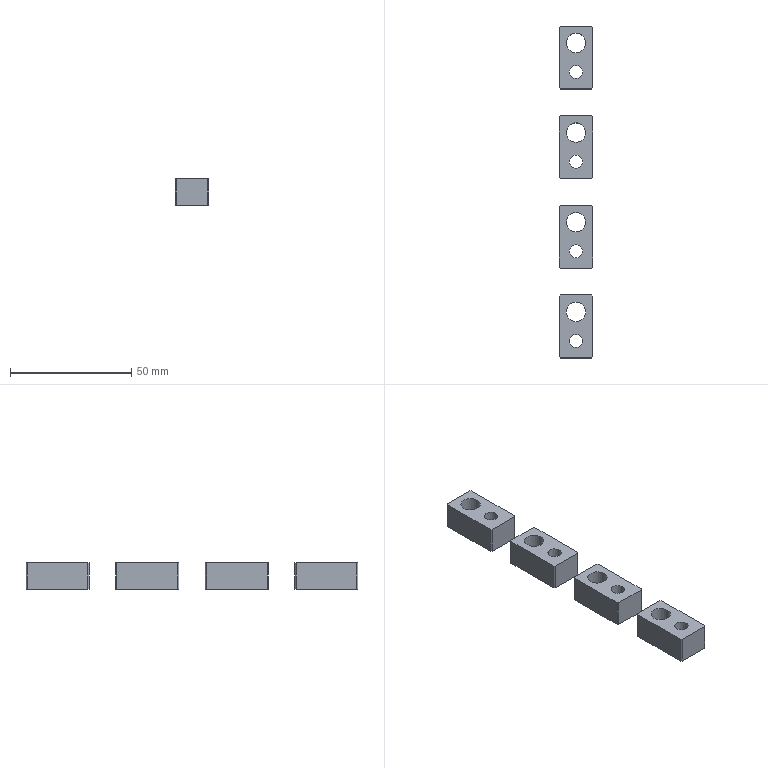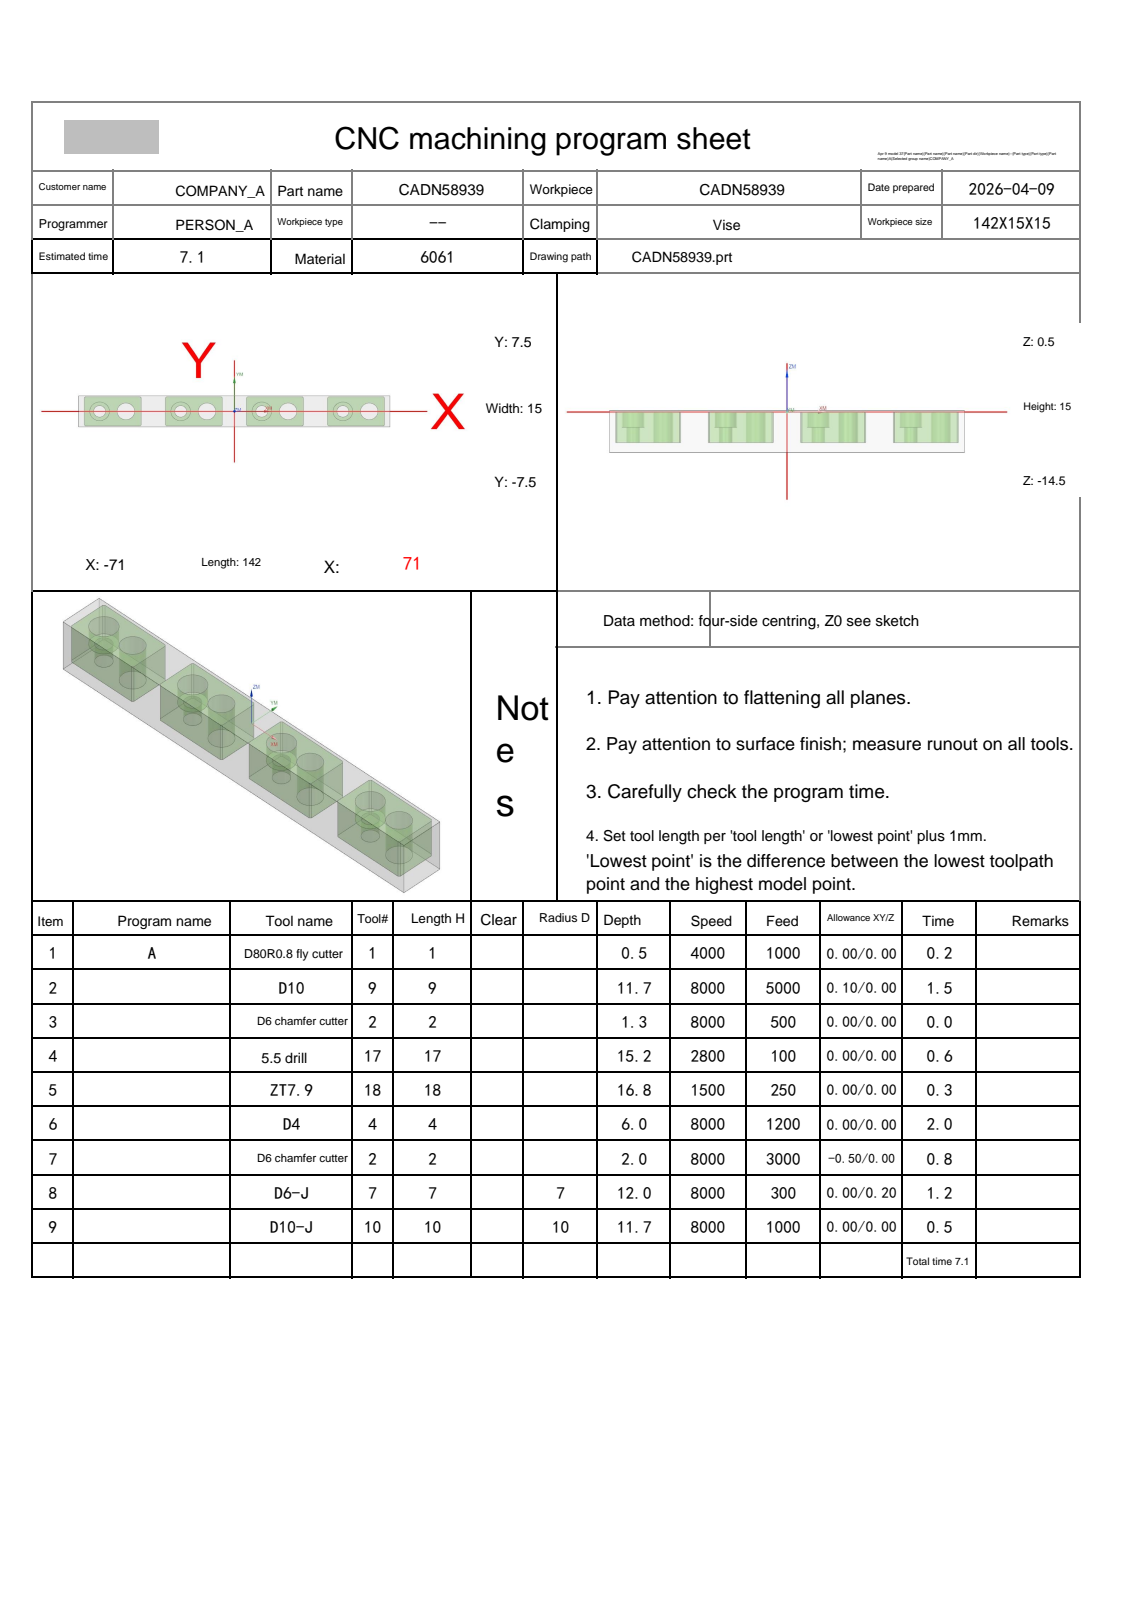NC program | NX | posted by the shop | part box 14 x 137 x 11 mm
Lines 1 to 1840 of 2072, first 1206 of 1838 lines:
%
O0001
(Machine time: 8.91 MIN)
(===Total Tool:8===)
(T1=D80R0.8 fly cutter D=80.  R=0.8  D-  H01 Z=-0.   )
(T9=D10     D=10.  R=0.   D-  H09 Z=-11.2 )
(T2=D6 chamfer cutter   D=6.   R=0.   D-  H02 Z=-1.5  )
(T17=5.5 drill  D=5.5  DR_a=118 D-  H17 Z=-14.65)
(T18=ZT7.9  D=7.9  DR_a=120 D-  H18 Z=-16.28)
(T4=D4      D=4.   R=0.   D4  H04 Z=-5.5  )
(T7=D6-J    D=6.   R=0.   D7  H07 Z=-11.5 )
(T10=D10-J  D=10.  R=0.   D10 H10 Z=-11.2 )
G80 G90 G17 G49 G40
G91 G28 Z0
M01
N1 T01 M06
(D80R0.8 fly cutter  D=80. R=0.8 H=01 ce=0.00 di=0.00)
G00 G90 G54 X-113.5 Y0.0 M03 S4000
G43 H01 Z20.
M08
Z2.
G01 Z0.0 F1000.
X-108.5
X108.5
X113.5
Z2.
G00 Z20.
G91 G28 Z0.0
M05
M09
G91 G28 Z0.0
M01
N2 T09 M06
(D10  D=10. R=0. H=09 ce=0.10 di=0.00)
G00 G90 G54 X18.5 Y12.1 M03 S8000
G43 H09 Z20.
M08
Z.5
G01 X31. Z.412 F5000.
G02 X34.606 Y10.606 Z.384 I0.0 J-5.1
G01 X35.106 Y10.106 Z.379
G02 X36.6 Y6.5 Z.351 I-3.606 J-3.606
G01 Y-6.5 Z.259
G02 X35.106 Y-10.106 Z.231 I-5.1 J0.0
G01 X34.606 Y-10.606 Z.226
G02 X31. Y-12.1 Z.198 I-3.606 J3.606
G01 X6. Z.022
G02 X2.394 Y-10.606 Z-.006 I0.0 J5.1
G01 X1.894 Y-10.106 Z-.011
G02 X.4 Y-6.5 Z-.039 I3.606 J3.606
G01 Y6.5 Z-.131
G02 X1.894 Y10.106 Z-.159 I5.1 J0.0
G01 X2.394 Y10.606 Z-.164
G02 X6. Y12.1 Z-.192 I3.606 J-3.606
G01 X31. Z-.368
G02 X34.606 Y10.606 Z-.396 I0.0 J-5.1
G01 X35.106 Y10.106 Z-.401
G02 X36.6 Y6.5 Z-.429 I-3.606 J-3.606
G01 Y-6.5 Z-.521
G02 X35.106 Y-10.106 Z-.549 I-5.1 J0.0
G01 X34.606 Y-10.606 Z-.554
G02 X31. Y-12.1 Z-.582 I-3.606 J3.606
G01 X6. Z-.758
G02 X2.394 Y-10.606 Z-.786 I0.0 J5.1
G01 X1.894 Y-10.106 Z-.791
G02 X.4 Y-6.5 Z-.819 I3.606 J3.606
G01 Y6.5 Z-.911
G02 X1.894 Y10.106 Z-.939 I5.1 J0.0
G01 X2.394 Y10.606 Z-.944
G02 X6. Y12.1 Z-.972 I3.606 J-3.606
G01 X31. Z-1.148
G02 X34.606 Y10.606 Z-1.176 I0.0 J-5.1
G01 X35.106 Y10.106 Z-1.181
G02 X36.6 Y6.5 Z-1.209 I-3.606 J-3.606
G01 Y-6.5 Z-1.301
G02 X35.106 Y-10.106 Z-1.329 I-5.1 J0.0
G01 X34.606 Y-10.606 Z-1.334
G02 X31. Y-12.1 Z-1.362 I-3.606 J3.606
G01 X6. Z-1.538
G02 X2.394 Y-10.606 Z-1.566 I0.0 J5.1
G01 X1.894 Y-10.106 Z-1.571
G02 X.4 Y-6.5 Z-1.599 I3.606 J3.606
G01 Y6.5 Z-1.691
G02 X1.894 Y10.106 Z-1.719 I5.1 J0.0
G01 X2.394 Y10.606 Z-1.724
G02 X6. Y12.1 Z-1.752 I3.606 J-3.606
G01 X31. Z-1.928
G02 X34.606 Y10.606 Z-1.956 I0.0 J-5.1
G01 X35.106 Y10.106 Z-1.961
G02 X36.6 Y6.5 Z-1.989 I-3.606 J-3.606
G01 Y-6.5 Z-2.081
G02 X35.106 Y-10.106 Z-2.109 I-5.1 J0.0
G01 X34.606 Y-10.606 Z-2.114
G02 X31. Y-12.1 Z-2.142 I-3.606 J3.606
G01 X6. Z-2.318
G02 X2.394 Y-10.606 Z-2.346 I0.0 J5.1
G01 X1.894 Y-10.106 Z-2.351
G02 X.4 Y-6.5 Z-2.379 I3.606 J3.606
G01 Y6.5 Z-2.471
G02 X1.894 Y10.106 Z-2.499 I5.1 J0.0
G01 X2.394 Y10.606 Z-2.504
G02 X6. Y12.1 Z-2.532 I3.606 J-3.606
G01 X31. Z-2.708
G02 X34.606 Y10.606 Z-2.736 I0.0 J-5.1
G01 X35.106 Y10.106 Z-2.741
G02 X36.6 Y6.5 Z-2.769 I-3.606 J-3.606
G01 Y-6.5 Z-2.861
G02 X35.106 Y-10.106 Z-2.889 I-5.1 J0.0
G01 X34.606 Y-10.606 Z-2.894
G02 X31. Y-12.1 Z-2.922 I-3.606 J3.606
G01 X6. Z-3.098
G02 X2.394 Y-10.606 Z-3.126 I0.0 J5.1
G01 X1.894 Y-10.106 Z-3.131
G02 X.4 Y-6.5 Z-3.159 I3.606 J3.606
G01 Y6.5 Z-3.251
G02 X1.894 Y10.106 Z-3.279 I5.1 J0.0
G01 X2.394 Y10.606 Z-3.284
G02 X6. Y12.1 Z-3.312 I3.606 J-3.606
G01 X31. Z-3.488
G02 X34.606 Y10.606 Z-3.516 I0.0 J-5.1
G01 X35.106 Y10.106 Z-3.521
G02 X36.6 Y6.5 Z-3.549 I-3.606 J-3.606
G01 Y-6.5 Z-3.641
G02 X35.106 Y-10.106 Z-3.669 I-5.1 J0.0
G01 X34.606 Y-10.606 Z-3.674
G02 X31. Y-12.1 Z-3.702 I-3.606 J3.606
G01 X6. Z-3.878
G02 X2.394 Y-10.606 Z-3.906 I0.0 J5.1
G01 X1.894 Y-10.106 Z-3.911
G02 X.4 Y-6.5 Z-3.939 I3.606 J3.606
G01 Y6.5 Z-4.031
G02 X1.894 Y10.106 Z-4.059 I5.1 J0.0
G01 X2.394 Y10.606 Z-4.064
G02 X6. Y12.1 Z-4.092 I3.606 J-3.606
G01 X31. Z-4.268
G02 X34.606 Y10.606 Z-4.296 I0.0 J-5.1
G01 X35.106 Y10.106 Z-4.301
G02 X36.6 Y6.5 Z-4.329 I-3.606 J-3.606
G01 Y-6.5 Z-4.421
G02 X35.106 Y-10.106 Z-4.449 I-5.1 J0.0
G01 X34.606 Y-10.606 Z-4.454
G02 X31. Y-12.1 Z-4.482 I-3.606 J3.606
G01 X6. Z-4.658
G02 X2.394 Y-10.606 Z-4.686 I0.0 J5.1
G01 X1.894 Y-10.106 Z-4.691
G02 X.4 Y-6.5 Z-4.719 I3.606 J3.606
G01 Y6.5 Z-4.811
G02 X1.894 Y10.106 Z-4.839 I5.1 J0.0
G01 X2.394 Y10.606 Z-4.844
G02 X6. Y12.1 Z-4.872 I3.606 J-3.606
G01 X31. Z-5.048
G02 X34.606 Y10.606 Z-5.076 I0.0 J-5.1
G01 X35.106 Y10.106 Z-5.081
G02 X36.6 Y6.5 Z-5.109 I-3.606 J-3.606
G01 Y-6.5 Z-5.201
G02 X35.106 Y-10.106 Z-5.229 I-5.1 J0.0
G01 X34.606 Y-10.606 Z-5.234
G02 X31. Y-12.1 Z-5.262 I-3.606 J3.606
G01 X6. Z-5.438
G02 X2.394 Y-10.606 Z-5.466 I0.0 J5.1
G01 X1.894 Y-10.106 Z-5.471
G02 X.4 Y-6.5 Z-5.499 I3.606 J3.606
G01 Y6.5 Z-5.591
G02 X1.894 Y10.106 Z-5.619 I5.1 J0.0
G01 X2.394 Y10.606 Z-5.624
G02 X6. Y12.1 Z-5.652 I3.606 J-3.606
G01 X31. Z-5.828
G02 X34.606 Y10.606 Z-5.856 I0.0 J-5.1
G01 X35.106 Y10.106 Z-5.861
G02 X36.6 Y6.5 Z-5.889 I-3.606 J-3.606
G01 Y-6.5 Z-5.981
G02 X35.106 Y-10.106 Z-6.009 I-5.1 J0.0
G01 X34.606 Y-10.606 Z-6.014
G02 X31. Y-12.1 Z-6.042 I-3.606 J3.606
G01 X6. Z-6.218
G02 X2.394 Y-10.606 Z-6.246 I0.0 J5.1
G01 X1.894 Y-10.106 Z-6.251
G02 X.4 Y-6.5 Z-6.279 I3.606 J3.606
G01 Y6.5 Z-6.371
G02 X1.894 Y10.106 Z-6.399 I5.1 J0.0
G01 X2.394 Y10.606 Z-6.404
G02 X6. Y12.1 Z-6.432 I3.606 J-3.606
G01 X31. Z-6.608
G02 X34.606 Y10.606 Z-6.636 I0.0 J-5.1
G01 X35.106 Y10.106 Z-6.641
G02 X36.6 Y6.5 Z-6.669 I-3.606 J-3.606
G01 Y-6.5 Z-6.761
G02 X35.106 Y-10.106 Z-6.789 I-5.1 J0.0
G01 X34.606 Y-10.606 Z-6.794
G02 X31. Y-12.1 Z-6.822 I-3.606 J3.606
G01 X6. Z-6.998
G02 X2.394 Y-10.606 Z-7.026 I0.0 J5.1
G01 X1.894 Y-10.106 Z-7.031
G02 X.4 Y-6.5 Z-7.059 I3.606 J3.606
G01 Y6.5 Z-7.151
G02 X1.894 Y10.106 Z-7.179 I5.1 J0.0
G01 X2.394 Y10.606 Z-7.184
G02 X6. Y12.1 Z-7.212 I3.606 J-3.606
G01 X31. Z-7.388
G02 X34.606 Y10.606 Z-7.416 I0.0 J-5.1
G01 X35.106 Y10.106 Z-7.421
G02 X36.6 Y6.5 Z-7.449 I-3.606 J-3.606
G01 Y-6.5 Z-7.541
G02 X35.106 Y-10.106 Z-7.569 I-5.1 J0.0
G01 X34.606 Y-10.606 Z-7.574
G02 X31. Y-12.1 Z-7.602 I-3.606 J3.606
G01 X6. Z-7.778
G02 X2.394 Y-10.606 Z-7.806 I0.0 J5.1
G01 X1.894 Y-10.106 Z-7.811
G02 X.4 Y-6.5 Z-7.839 I3.606 J3.606
G01 Y6.5 Z-7.931
G02 X1.894 Y10.106 Z-7.959 I5.1 J0.0
G01 X2.394 Y10.606 Z-7.964
G02 X6. Y12.1 Z-7.992 I3.606 J-3.606
G01 X31. Z-8.168
G02 X34.606 Y10.606 Z-8.196 I0.0 J-5.1
G01 X35.106 Y10.106 Z-8.201
G02 X36.6 Y6.5 Z-8.229 I-3.606 J-3.606
G01 Y-6.5 Z-8.321
G02 X35.106 Y-10.106 Z-8.349 I-5.1 J0.0
G01 X34.606 Y-10.606 Z-8.354
G02 X31. Y-12.1 Z-8.382 I-3.606 J3.606
G01 X6. Z-8.558
G02 X2.394 Y-10.606 Z-8.586 I0.0 J5.1
G01 X1.894 Y-10.106 Z-8.591
G02 X.4 Y-6.5 Z-8.619 I3.606 J3.606
G01 Y6.5 Z-8.711
G02 X1.894 Y10.106 Z-8.739 I5.1 J0.0
G01 X2.394 Y10.606 Z-8.744
G02 X6. Y12.1 Z-8.772 I3.606 J-3.606
G01 X31. Z-8.948
G02 X34.606 Y10.606 Z-8.976 I0.0 J-5.1
G01 X35.106 Y10.106 Z-8.981
G02 X36.6 Y6.5 Z-9.009 I-3.606 J-3.606
G01 Y-6.5 Z-9.101
G02 X35.106 Y-10.106 Z-9.129 I-5.1 J0.0
G01 X34.606 Y-10.606 Z-9.134
G02 X31. Y-12.1 Z-9.162 I-3.606 J3.606
G01 X6. Z-9.338
G02 X2.394 Y-10.606 Z-9.366 I0.0 J5.1
G01 X1.894 Y-10.106 Z-9.371
G02 X.4 Y-6.5 Z-9.399 I3.606 J3.606
G01 Y6.5 Z-9.491
G02 X1.894 Y10.106 Z-9.519 I5.1 J0.0
G01 X2.394 Y10.606 Z-9.524
G02 X6. Y12.1 Z-9.552 I3.606 J-3.606
G01 X31. Z-9.728
G02 X34.606 Y10.606 Z-9.756 I0.0 J-5.1
G01 X35.106 Y10.106 Z-9.761
G02 X36.6 Y6.5 Z-9.789 I-3.606 J-3.606
G01 Y-6.5 Z-9.881
G02 X35.106 Y-10.106 Z-9.909 I-5.1 J0.0
G01 X34.606 Y-10.606 Z-9.914
G02 X31. Y-12.1 Z-9.942 I-3.606 J3.606
G01 X6. Z-10.118
G02 X2.394 Y-10.606 Z-10.146 I0.0 J5.1
G01 X1.894 Y-10.106 Z-10.151
G02 X.4 Y-6.5 Z-10.179 I3.606 J3.606
G01 Y6.5 Z-10.271
G02 X1.894 Y10.106 Z-10.299 I5.1 J0.0
G01 X2.394 Y10.606 Z-10.304
G02 X6. Y12.1 Z-10.332 I3.606 J-3.606
G01 X31. Z-10.508
G02 X34.606 Y10.606 Z-10.536 I0.0 J-5.1
G01 X35.106 Y10.106 Z-10.541
G02 X36.6 Y6.5 Z-10.569 I-3.606 J-3.606
G01 Y-6.5 Z-10.661
G02 X35.106 Y-10.106 Z-10.689 I-5.1 J0.0
G01 X34.606 Y-10.606 Z-10.694
G02 X31. Y-12.1 Z-10.722 I-3.606 J3.606
G01 X6. Z-10.898
G02 X2.394 Y-10.606 Z-10.926 I0.0 J5.1
G01 X1.894 Y-10.106 Z-10.931
G02 X.4 Y-6.5 Z-10.959 I3.606 J3.606
G01 Y6.5 Z-11.051
G02 X1.894 Y10.106 Z-11.079 I5.1 J0.0
G01 X2.394 Y10.606 Z-11.084
G02 X6. Y12.1 Z-11.112 I3.606 J-3.606
G01 X18.5 Z-11.2
X31.
G02 X34.606 Y10.606 I0.0 J-5.1
G01 X35.106 Y10.106
G02 X36.6 Y6.5 I-3.606 J-3.606
G01 Y-6.5
G02 X35.106 Y-10.106 I-5.1 J0.0
G01 X34.606 Y-10.606
G02 X31. Y-12.1 I-3.606 J3.606
G01 X6.
G02 X2.394 Y-10.606 I0.0 J5.1
G01 X1.894 Y-10.106
G02 X.4 Y-6.5 I3.606 J3.606
G01 Y6.5
G02 X1.894 Y10.106 I5.1 J0.0
G01 X2.394 Y10.606
G02 X6. Y12.1 I3.606 J-3.606
G01 X18.5
X19.
Z-10.2
G00 Z20.
X-18.5
Z.5
G01 X-6. Z.412
G02 X-2.394 Y10.606 Z.384 I0.0 J-5.1
G01 X-1.894 Y10.106 Z.379
G02 X-.4 Y6.5 Z.351 I-3.606 J-3.606
G01 Y-6.5 Z.259
G02 X-1.894 Y-10.106 Z.231 I-5.1 J0.0
G01 X-2.394 Y-10.606 Z.226
G02 X-6. Y-12.1 Z.198 I-3.606 J3.606
G01 X-31. Z.022
G02 X-34.606 Y-10.606 Z-.006 I0.0 J5.1
G01 X-35.106 Y-10.106 Z-.011
G02 X-36.6 Y-6.5 Z-.039 I3.606 J3.606
G01 Y6.5 Z-.131
G02 X-35.106 Y10.106 Z-.159 I5.1 J0.0
G01 X-34.606 Y10.606 Z-.164
G02 X-31. Y12.1 Z-.192 I3.606 J-3.606
G01 X-6. Z-.368
G02 X-2.394 Y10.606 Z-.396 I0.0 J-5.1
G01 X-1.894 Y10.106 Z-.401
G02 X-.4 Y6.5 Z-.429 I-3.606 J-3.606
G01 Y-6.5 Z-.521
G02 X-1.894 Y-10.106 Z-.549 I-5.1 J0.0
G01 X-2.394 Y-10.606 Z-.554
G02 X-6. Y-12.1 Z-.582 I-3.606 J3.606
G01 X-31. Z-.758
G02 X-34.606 Y-10.606 Z-.786 I0.0 J5.1
G01 X-35.106 Y-10.106 Z-.791
G02 X-36.6 Y-6.5 Z-.819 I3.606 J3.606
G01 Y6.5 Z-.911
G02 X-35.106 Y10.106 Z-.939 I5.1 J0.0
G01 X-34.606 Y10.606 Z-.944
G02 X-31. Y12.1 Z-.972 I3.606 J-3.606
G01 X-6. Z-1.148
G02 X-2.394 Y10.606 Z-1.176 I0.0 J-5.1
G01 X-1.894 Y10.106 Z-1.181
G02 X-.4 Y6.5 Z-1.209 I-3.606 J-3.606
G01 Y-6.5 Z-1.301
G02 X-1.894 Y-10.106 Z-1.329 I-5.1 J0.0
G01 X-2.394 Y-10.606 Z-1.334
G02 X-6. Y-12.1 Z-1.362 I-3.606 J3.606
G01 X-31. Z-1.538
G02 X-34.606 Y-10.606 Z-1.566 I0.0 J5.1
G01 X-35.106 Y-10.106 Z-1.571
G02 X-36.6 Y-6.5 Z-1.599 I3.606 J3.606
G01 Y6.5 Z-1.691
G02 X-35.106 Y10.106 Z-1.719 I5.1 J0.0
G01 X-34.606 Y10.606 Z-1.724
G02 X-31. Y12.1 Z-1.752 I3.606 J-3.606
G01 X-6. Z-1.928
G02 X-2.394 Y10.606 Z-1.956 I0.0 J-5.1
G01 X-1.894 Y10.106 Z-1.961
G02 X-.4 Y6.5 Z-1.989 I-3.606 J-3.606
G01 Y-6.5 Z-2.081
G02 X-1.894 Y-10.106 Z-2.109 I-5.1 J0.0
G01 X-2.394 Y-10.606 Z-2.114
G02 X-6. Y-12.1 Z-2.142 I-3.606 J3.606
G01 X-31. Z-2.318
G02 X-34.606 Y-10.606 Z-2.346 I0.0 J5.1
G01 X-35.106 Y-10.106 Z-2.351
G02 X-36.6 Y-6.5 Z-2.379 I3.606 J3.606
G01 Y6.5 Z-2.471
G02 X-35.106 Y10.106 Z-2.499 I5.1 J0.0
G01 X-34.606 Y10.606 Z-2.504
G02 X-31. Y12.1 Z-2.532 I3.606 J-3.606
G01 X-6. Z-2.708
G02 X-2.394 Y10.606 Z-2.736 I0.0 J-5.1
G01 X-1.894 Y10.106 Z-2.741
G02 X-.4 Y6.5 Z-2.769 I-3.606 J-3.606
G01 Y-6.5 Z-2.861
G02 X-1.894 Y-10.106 Z-2.889 I-5.1 J0.0
G01 X-2.394 Y-10.606 Z-2.894
G02 X-6. Y-12.1 Z-2.922 I-3.606 J3.606
G01 X-31. Z-3.098
G02 X-34.606 Y-10.606 Z-3.126 I0.0 J5.1
G01 X-35.106 Y-10.106 Z-3.131
G02 X-36.6 Y-6.5 Z-3.159 I3.606 J3.606
G01 Y6.5 Z-3.251
G02 X-35.106 Y10.106 Z-3.279 I5.1 J0.0
G01 X-34.606 Y10.606 Z-3.284
G02 X-31. Y12.1 Z-3.312 I3.606 J-3.606
G01 X-6. Z-3.488
G02 X-2.394 Y10.606 Z-3.516 I0.0 J-5.1
G01 X-1.894 Y10.106 Z-3.521
G02 X-.4 Y6.5 Z-3.549 I-3.606 J-3.606
G01 Y-6.5 Z-3.641
G02 X-1.894 Y-10.106 Z-3.669 I-5.1 J0.0
G01 X-2.394 Y-10.606 Z-3.674
G02 X-6. Y-12.1 Z-3.702 I-3.606 J3.606
G01 X-31. Z-3.878
G02 X-34.606 Y-10.606 Z-3.906 I0.0 J5.1
G01 X-35.106 Y-10.106 Z-3.911
G02 X-36.6 Y-6.5 Z-3.939 I3.606 J3.606
G01 Y6.5 Z-4.031
G02 X-35.106 Y10.106 Z-4.059 I5.1 J0.0
G01 X-34.606 Y10.606 Z-4.064
G02 X-31. Y12.1 Z-4.092 I3.606 J-3.606
G01 X-6. Z-4.268
G02 X-2.394 Y10.606 Z-4.296 I0.0 J-5.1
G01 X-1.894 Y10.106 Z-4.301
G02 X-.4 Y6.5 Z-4.329 I-3.606 J-3.606
G01 Y-6.5 Z-4.421
G02 X-1.894 Y-10.106 Z-4.449 I-5.1 J0.0
G01 X-2.394 Y-10.606 Z-4.454
G02 X-6. Y-12.1 Z-4.482 I-3.606 J3.606
G01 X-31. Z-4.658
G02 X-34.606 Y-10.606 Z-4.686 I0.0 J5.1
G01 X-35.106 Y-10.106 Z-4.691
G02 X-36.6 Y-6.5 Z-4.719 I3.606 J3.606
G01 Y6.5 Z-4.811
G02 X-35.106 Y10.106 Z-4.839 I5.1 J0.0
G01 X-34.606 Y10.606 Z-4.844
G02 X-31. Y12.1 Z-4.872 I3.606 J-3.606
G01 X-6. Z-5.048
G02 X-2.394 Y10.606 Z-5.076 I0.0 J-5.1
G01 X-1.894 Y10.106 Z-5.081
G02 X-.4 Y6.5 Z-5.109 I-3.606 J-3.606
G01 Y-6.5 Z-5.201
G02 X-1.894 Y-10.106 Z-5.229 I-5.1 J0.0
G01 X-2.394 Y-10.606 Z-5.234
G02 X-6. Y-12.1 Z-5.262 I-3.606 J3.606
G01 X-31. Z-5.438
G02 X-34.606 Y-10.606 Z-5.466 I0.0 J5.1
G01 X-35.106 Y-10.106 Z-5.471
G02 X-36.6 Y-6.5 Z-5.499 I3.606 J3.606
G01 Y6.5 Z-5.591
G02 X-35.106 Y10.106 Z-5.619 I5.1 J0.0
G01 X-34.606 Y10.606 Z-5.624
G02 X-31. Y12.1 Z-5.652 I3.606 J-3.606
G01 X-6. Z-5.828
G02 X-2.394 Y10.606 Z-5.856 I0.0 J-5.1
G01 X-1.894 Y10.106 Z-5.861
G02 X-.4 Y6.5 Z-5.889 I-3.606 J-3.606
G01 Y-6.5 Z-5.981
G02 X-1.894 Y-10.106 Z-6.009 I-5.1 J0.0
G01 X-2.394 Y-10.606 Z-6.014
G02 X-6. Y-12.1 Z-6.042 I-3.606 J3.606
G01 X-31. Z-6.218
G02 X-34.606 Y-10.606 Z-6.246 I0.0 J5.1
G01 X-35.106 Y-10.106 Z-6.251
G02 X-36.6 Y-6.5 Z-6.279 I3.606 J3.606
G01 Y6.5 Z-6.371
G02 X-35.106 Y10.106 Z-6.399 I5.1 J0.0
G01 X-34.606 Y10.606 Z-6.404
G02 X-31. Y12.1 Z-6.432 I3.606 J-3.606
G01 X-6. Z-6.608
G02 X-2.394 Y10.606 Z-6.636 I0.0 J-5.1
G01 X-1.894 Y10.106 Z-6.641
G02 X-.4 Y6.5 Z-6.669 I-3.606 J-3.606
G01 Y-6.5 Z-6.761
G02 X-1.894 Y-10.106 Z-6.789 I-5.1 J0.0
G01 X-2.394 Y-10.606 Z-6.794
G02 X-6. Y-12.1 Z-6.822 I-3.606 J3.606
G01 X-31. Z-6.998
G02 X-34.606 Y-10.606 Z-7.026 I0.0 J5.1
G01 X-35.106 Y-10.106 Z-7.031
G02 X-36.6 Y-6.5 Z-7.059 I3.606 J3.606
G01 Y6.5 Z-7.151
G02 X-35.106 Y10.106 Z-7.179 I5.1 J0.0
G01 X-34.606 Y10.606 Z-7.184
G02 X-31. Y12.1 Z-7.212 I3.606 J-3.606
G01 X-6. Z-7.388
G02 X-2.394 Y10.606 Z-7.416 I0.0 J-5.1
G01 X-1.894 Y10.106 Z-7.421
G02 X-.4 Y6.5 Z-7.449 I-3.606 J-3.606
G01 Y-6.5 Z-7.541
G02 X-1.894 Y-10.106 Z-7.569 I-5.1 J0.0
G01 X-2.394 Y-10.606 Z-7.574
G02 X-6. Y-12.1 Z-7.602 I-3.606 J3.606
G01 X-31. Z-7.778
G02 X-34.606 Y-10.606 Z-7.806 I0.0 J5.1
G01 X-35.106 Y-10.106 Z-7.811
G02 X-36.6 Y-6.5 Z-7.839 I3.606 J3.606
G01 Y6.5 Z-7.931
G02 X-35.106 Y10.106 Z-7.959 I5.1 J0.0
G01 X-34.606 Y10.606 Z-7.964
G02 X-31. Y12.1 Z-7.992 I3.606 J-3.606
G01 X-6. Z-8.168
G02 X-2.394 Y10.606 Z-8.196 I0.0 J-5.1
G01 X-1.894 Y10.106 Z-8.201
G02 X-.4 Y6.5 Z-8.229 I-3.606 J-3.606
G01 Y-6.5 Z-8.321
G02 X-1.894 Y-10.106 Z-8.349 I-5.1 J0.0
G01 X-2.394 Y-10.606 Z-8.354
G02 X-6. Y-12.1 Z-8.382 I-3.606 J3.606
G01 X-31. Z-8.558
G02 X-34.606 Y-10.606 Z-8.586 I0.0 J5.1
G01 X-35.106 Y-10.106 Z-8.591
G02 X-36.6 Y-6.5 Z-8.619 I3.606 J3.606
G01 Y6.5 Z-8.711
G02 X-35.106 Y10.106 Z-8.739 I5.1 J0.0
G01 X-34.606 Y10.606 Z-8.744
G02 X-31. Y12.1 Z-8.772 I3.606 J-3.606
G01 X-6. Z-8.948
G02 X-2.394 Y10.606 Z-8.976 I0.0 J-5.1
G01 X-1.894 Y10.106 Z-8.981
G02 X-.4 Y6.5 Z-9.009 I-3.606 J-3.606
G01 Y-6.5 Z-9.101
G02 X-1.894 Y-10.106 Z-9.129 I-5.1 J0.0
G01 X-2.394 Y-10.606 Z-9.134
G02 X-6. Y-12.1 Z-9.162 I-3.606 J3.606
G01 X-31. Z-9.338
G02 X-34.606 Y-10.606 Z-9.366 I0.0 J5.1
G01 X-35.106 Y-10.106 Z-9.371
G02 X-36.6 Y-6.5 Z-9.399 I3.606 J3.606
G01 Y6.5 Z-9.491
G02 X-35.106 Y10.106 Z-9.519 I5.1 J0.0
G01 X-34.606 Y10.606 Z-9.524
G02 X-31. Y12.1 Z-9.552 I3.606 J-3.606
G01 X-6. Z-9.728
G02 X-2.394 Y10.606 Z-9.756 I0.0 J-5.1
G01 X-1.894 Y10.106 Z-9.761
G02 X-.4 Y6.5 Z-9.789 I-3.606 J-3.606
G01 Y-6.5 Z-9.881
G02 X-1.894 Y-10.106 Z-9.909 I-5.1 J0.0
G01 X-2.394 Y-10.606 Z-9.914
G02 X-6. Y-12.1 Z-9.942 I-3.606 J3.606
G01 X-31. Z-10.118
G02 X-34.606 Y-10.606 Z-10.146 I0.0 J5.1
G01 X-35.106 Y-10.106 Z-10.151
G02 X-36.6 Y-6.5 Z-10.179 I3.606 J3.606
G01 Y6.5 Z-10.271
G02 X-35.106 Y10.106 Z-10.299 I5.1 J0.0
G01 X-34.606 Y10.606 Z-10.304
G02 X-31. Y12.1 Z-10.332 I3.606 J-3.606
G01 X-6. Z-10.508
G02 X-2.394 Y10.606 Z-10.536 I0.0 J-5.1
G01 X-1.894 Y10.106 Z-10.541
G02 X-.4 Y6.5 Z-10.569 I-3.606 J-3.606
G01 Y-6.5 Z-10.661
G02 X-1.894 Y-10.106 Z-10.689 I-5.1 J0.0
G01 X-2.394 Y-10.606 Z-10.694
G02 X-6. Y-12.1 Z-10.722 I-3.606 J3.606
G01 X-31. Z-10.898
G02 X-34.606 Y-10.606 Z-10.926 I0.0 J5.1
G01 X-35.106 Y-10.106 Z-10.931
G02 X-36.6 Y-6.5 Z-10.959 I3.606 J3.606
G01 Y6.5 Z-11.051
G02 X-35.106 Y10.106 Z-11.079 I5.1 J0.0
G01 X-34.606 Y10.606 Z-11.084
G02 X-31. Y12.1 Z-11.112 I3.606 J-3.606
G01 X-18.5 Z-11.2
X-6.
G02 X-2.394 Y10.606 I0.0 J-5.1
G01 X-1.894 Y10.106
G02 X-.4 Y6.5 I-3.606 J-3.606
G01 Y-6.5
G02 X-1.894 Y-10.106 I-5.1 J0.0
G01 X-2.394 Y-10.606
G02 X-6. Y-12.1 I-3.606 J3.606
G01 X-31.
G02 X-34.606 Y-10.606 I0.0 J5.1
G01 X-35.106 Y-10.106
G02 X-36.6 Y-6.5 I3.606 J3.606
G01 Y6.5
G02 X-35.106 Y10.106 I5.1 J0.0
G01 X-34.606 Y10.606
G02 X-31. Y12.1 I3.606 J-3.606
G01 X-18.5
X-18.
Z-10.2
G00 Z20.
X-55.5
Z.5
G01 X-43. Z.412
G02 X-39.394 Y10.606 Z.384 I0.0 J-5.1
G01 X-38.894 Y10.106 Z.379
G02 X-37.4 Y6.5 Z.351 I-3.606 J-3.606
G01 Y-6.5 Z.259
G02 X-38.894 Y-10.106 Z.231 I-5.1 J0.0
G01 X-39.394 Y-10.606 Z.226
G02 X-43. Y-12.1 Z.198 I-3.606 J3.606
G01 X-68. Z.022
G02 X-71.606 Y-10.606 Z-.006 I0.0 J5.1
G01 X-72.106 Y-10.106 Z-.011
G02 X-73.6 Y-6.5 Z-.039 I3.606 J3.606
G01 Y6.5 Z-.131
G02 X-72.106 Y10.106 Z-.159 I5.1 J0.0
G01 X-71.606 Y10.606 Z-.164
G02 X-68. Y12.1 Z-.192 I3.606 J-3.606
G01 X-43. Z-.368
G02 X-39.394 Y10.606 Z-.396 I0.0 J-5.1
G01 X-38.894 Y10.106 Z-.401
G02 X-37.4 Y6.5 Z-.429 I-3.606 J-3.606
G01 Y-6.5 Z-.521
G02 X-38.894 Y-10.106 Z-.549 I-5.1 J0.0
G01 X-39.394 Y-10.606 Z-.554
G02 X-43. Y-12.1 Z-.582 I-3.606 J3.606
G01 X-68. Z-.758
G02 X-71.606 Y-10.606 Z-.786 I0.0 J5.1
G01 X-72.106 Y-10.106 Z-.791
G02 X-73.6 Y-6.5 Z-.819 I3.606 J3.606
G01 Y6.5 Z-.911
G02 X-72.106 Y10.106 Z-.939 I5.1 J0.0
G01 X-71.606 Y10.606 Z-.944
G02 X-68. Y12.1 Z-.972 I3.606 J-3.606
G01 X-43. Z-1.148
G02 X-39.394 Y10.606 Z-1.176 I0.0 J-5.1
G01 X-38.894 Y10.106 Z-1.181
G02 X-37.4 Y6.5 Z-1.209 I-3.606 J-3.606
G01 Y-6.5 Z-1.301
G02 X-38.894 Y-10.106 Z-1.329 I-5.1 J0.0
G01 X-39.394 Y-10.606 Z-1.334
G02 X-43. Y-12.1 Z-1.362 I-3.606 J3.606
G01 X-68. Z-1.538
G02 X-71.606 Y-10.606 Z-1.566 I0.0 J5.1
G01 X-72.106 Y-10.106 Z-1.571
G02 X-73.6 Y-6.5 Z-1.599 I3.606 J3.606
G01 Y6.5 Z-1.691
G02 X-72.106 Y10.106 Z-1.719 I5.1 J0.0
G01 X-71.606 Y10.606 Z-1.724
G02 X-68. Y12.1 Z-1.752 I3.606 J-3.606
G01 X-43. Z-1.928
G02 X-39.394 Y10.606 Z-1.956 I0.0 J-5.1
G01 X-38.894 Y10.106 Z-1.961
G02 X-37.4 Y6.5 Z-1.989 I-3.606 J-3.606
G01 Y-6.5 Z-2.081
G02 X-38.894 Y-10.106 Z-2.109 I-5.1 J0.0
G01 X-39.394 Y-10.606 Z-2.114
G02 X-43. Y-12.1 Z-2.142 I-3.606 J3.606
G01 X-68. Z-2.318
G02 X-71.606 Y-10.606 Z-2.346 I0.0 J5.1
G01 X-72.106 Y-10.106 Z-2.351
G02 X-73.6 Y-6.5 Z-2.379 I3.606 J3.606
G01 Y6.5 Z-2.471
G02 X-72.106 Y10.106 Z-2.499 I5.1 J0.0
G01 X-71.606 Y10.606 Z-2.504
G02 X-68. Y12.1 Z-2.532 I3.606 J-3.606
G01 X-43. Z-2.708
G02 X-39.394 Y10.606 Z-2.736 I0.0 J-5.1
G01 X-38.894 Y10.106 Z-2.741
G02 X-37.4 Y6.5 Z-2.769 I-3.606 J-3.606
G01 Y-6.5 Z-2.861
G02 X-38.894 Y-10.106 Z-2.889 I-5.1 J0.0
G01 X-39.394 Y-10.606 Z-2.894
G02 X-43. Y-12.1 Z-2.922 I-3.606 J3.606
G01 X-68. Z-3.098
G02 X-71.606 Y-10.606 Z-3.126 I0.0 J5.1
G01 X-72.106 Y-10.106 Z-3.131
G02 X-73.6 Y-6.5 Z-3.159 I3.606 J3.606
G01 Y6.5 Z-3.251
G02 X-72.106 Y10.106 Z-3.279 I5.1 J0.0
G01 X-71.606 Y10.606 Z-3.284
G02 X-68. Y12.1 Z-3.312 I3.606 J-3.606
G01 X-43. Z-3.488
G02 X-39.394 Y10.606 Z-3.516 I0.0 J-5.1
G01 X-38.894 Y10.106 Z-3.521
G02 X-37.4 Y6.5 Z-3.549 I-3.606 J-3.606
G01 Y-6.5 Z-3.641
G02 X-38.894 Y-10.106 Z-3.669 I-5.1 J0.0
G01 X-39.394 Y-10.606 Z-3.674
G02 X-43. Y-12.1 Z-3.702 I-3.606 J3.606
G01 X-68. Z-3.878
G02 X-71.606 Y-10.606 Z-3.906 I0.0 J5.1
G01 X-72.106 Y-10.106 Z-3.911
G02 X-73.6 Y-6.5 Z-3.939 I3.606 J3.606
G01 Y6.5 Z-4.031
G02 X-72.106 Y10.106 Z-4.059 I5.1 J0.0
G01 X-71.606 Y10.606 Z-4.064
G02 X-68. Y12.1 Z-4.092 I3.606 J-3.606
G01 X-43. Z-4.268
G02 X-39.394 Y10.606 Z-4.296 I0.0 J-5.1
G01 X-38.894 Y10.106 Z-4.301
G02 X-37.4 Y6.5 Z-4.329 I-3.606 J-3.606
G01 Y-6.5 Z-4.421
G02 X-38.894 Y-10.106 Z-4.449 I-5.1 J0.0
G01 X-39.394 Y-10.606 Z-4.454
G02 X-43. Y-12.1 Z-4.482 I-3.606 J3.606
G01 X-68. Z-4.658
G02 X-71.606 Y-10.606 Z-4.686 I0.0 J5.1
G01 X-72.106 Y-10.106 Z-4.691
G02 X-73.6 Y-6.5 Z-4.719 I3.606 J3.606
G01 Y6.5 Z-4.811
G02 X-72.106 Y10.106 Z-4.839 I5.1 J0.0
G01 X-71.606 Y10.606 Z-4.844
G02 X-68. Y12.1 Z-4.872 I3.606 J-3.606
G01 X-43. Z-5.048
G02 X-39.394 Y10.606 Z-5.076 I0.0 J-5.1
G01 X-38.894 Y10.106 Z-5.081
G02 X-37.4 Y6.5 Z-5.109 I-3.606 J-3.606
G01 Y-6.5 Z-5.201
G02 X-38.894 Y-10.106 Z-5.229 I-5.1 J0.0
G01 X-39.394 Y-10.606 Z-5.234
G02 X-43. Y-12.1 Z-5.262 I-3.606 J3.606
G01 X-68. Z-5.438
G02 X-71.606 Y-10.606 Z-5.466 I0.0 J5.1
G01 X-72.106 Y-10.106 Z-5.471
G02 X-73.6 Y-6.5 Z-5.499 I3.606 J3.606
G01 Y6.5 Z-5.591
G02 X-72.106 Y10.106 Z-5.619 I5.1 J0.0
G01 X-71.606 Y10.606 Z-5.624
G02 X-68. Y12.1 Z-5.652 I3.606 J-3.606
G01 X-43. Z-5.828
G02 X-39.394 Y10.606 Z-5.856 I0.0 J-5.1
G01 X-38.894 Y10.106 Z-5.861
G02 X-37.4 Y6.5 Z-5.889 I-3.606 J-3.606
G01 Y-6.5 Z-5.981
G02 X-38.894 Y-10.106 Z-6.009 I-5.1 J0.0
G01 X-39.394 Y-10.606 Z-6.014
G02 X-43. Y-12.1 Z-6.042 I-3.606 J3.606
G01 X-68. Z-6.218
G02 X-71.606 Y-10.606 Z-6.246 I0.0 J5.1
G01 X-72.106 Y-10.106 Z-6.251
G02 X-73.6 Y-6.5 Z-6.279 I3.606 J3.606
G01 Y6.5 Z-6.371
G02 X-72.106 Y10.106 Z-6.399 I5.1 J0.0
G01 X-71.606 Y10.606 Z-6.404
G02 X-68. Y12.1 Z-6.432 I3.606 J-3.606
G01 X-43. Z-6.608
G02 X-39.394 Y10.606 Z-6.636 I0.0 J-5.1
G01 X-38.894 Y10.106 Z-6.641
G02 X-37.4 Y6.5 Z-6.669 I-3.606 J-3.606
G01 Y-6.5 Z-6.761
G02 X-38.894 Y-10.106 Z-6.789 I-5.1 J0.0
G01 X-39.394 Y-10.606 Z-6.794
G02 X-43. Y-12.1 Z-6.822 I-3.606 J3.606
G01 X-68. Z-6.998
G02 X-71.606 Y-10.606 Z-7.026 I0.0 J5.1
G01 X-72.106 Y-10.106 Z-7.031
G02 X-73.6 Y-6.5 Z-7.059 I3.606 J3.606
G01 Y6.5 Z-7.151
G02 X-72.106 Y10.106 Z-7.179 I5.1 J0.0
G01 X-71.606 Y10.606 Z-7.184
G02 X-68. Y12.1 Z-7.212 I3.606 J-3.606
G01 X-43. Z-7.388
G02 X-39.394 Y10.606 Z-7.416 I0.0 J-5.1
G01 X-38.894 Y10.106 Z-7.421
G02 X-37.4 Y6.5 Z-7.449 I-3.606 J-3.606
G01 Y-6.5 Z-7.541
G02 X-38.894 Y-10.106 Z-7.569 I-5.1 J0.0
G01 X-39.394 Y-10.606 Z-7.574
G02 X-43. Y-12.1 Z-7.602 I-3.606 J3.606
G01 X-68. Z-7.778
G02 X-71.606 Y-10.606 Z-7.806 I0.0 J5.1
G01 X-72.106 Y-10.106 Z-7.811
G02 X-73.6 Y-6.5 Z-7.839 I3.606 J3.606
G01 Y6.5 Z-7.931
G02 X-72.106 Y10.106 Z-7.959 I5.1 J0.0
G01 X-71.606 Y10.606 Z-7.964
G02 X-68. Y12.1 Z-7.992 I3.606 J-3.606
G01 X-43. Z-8.168
G02 X-39.394 Y10.606 Z-8.196 I0.0 J-5.1
G01 X-38.894 Y10.106 Z-8.201
G02 X-37.4 Y6.5 Z-8.229 I-3.606 J-3.606
G01 Y-6.5 Z-8.321
G02 X-38.894 Y-10.106 Z-8.349 I-5.1 J0.0
G01 X-39.394 Y-10.606 Z-8.354
G02 X-43. Y-12.1 Z-8.382 I-3.606 J3.606
G01 X-68. Z-8.558
G02 X-71.606 Y-10.606 Z-8.586 I0.0 J5.1
G01 X-72.106 Y-10.106 Z-8.591
G02 X-73.6 Y-6.5 Z-8.619 I3.606 J3.606
G01 Y6.5 Z-8.711
G02 X-72.106 Y10.106 Z-8.739 I5.1 J0.0
G01 X-71.606 Y10.606 Z-8.744
G02 X-68. Y12.1 Z-8.772 I3.606 J-3.606
G01 X-43. Z-8.948
G02 X-39.394 Y10.606 Z-8.976 I0.0 J-5.1
G01 X-38.894 Y10.106 Z-8.981
G02 X-37.4 Y6.5 Z-9.009 I-3.606 J-3.606
G01 Y-6.5 Z-9.101
G02 X-38.894 Y-10.106 Z-9.129 I-5.1 J0.0
G01 X-39.394 Y-10.606 Z-9.134
G02 X-43. Y-12.1 Z-9.162 I-3.606 J3.606
G01 X-68. Z-9.338
G02 X-71.606 Y-10.606 Z-9.366 I0.0 J5.1
G01 X-72.106 Y-10.106 Z-9.371
G02 X-73.6 Y-6.5 Z-9.399 I3.606 J3.606
G01 Y6.5 Z-9.491
G02 X-72.106 Y10.106 Z-9.519 I5.1 J0.0
G01 X-71.606 Y10.606 Z-9.524
G02 X-68. Y12.1 Z-9.552 I3.606 J-3.606
G01 X-43. Z-9.728
G02 X-39.394 Y10.606 Z-9.756 I0.0 J-5.1
G01 X-38.894 Y10.106 Z-9.761
G02 X-37.4 Y6.5 Z-9.789 I-3.606 J-3.606
G01 Y-6.5 Z-9.881
G02 X-38.894 Y-10.106 Z-9.909 I-5.1 J0.0
G01 X-39.394 Y-10.606 Z-9.914
G02 X-43. Y-12.1 Z-9.942 I-3.606 J3.606
G01 X-68. Z-10.118
G02 X-71.606 Y-10.606 Z-10.146 I0.0 J5.1
G01 X-72.106 Y-10.106 Z-10.151
G02 X-73.6 Y-6.5 Z-10.179 I3.606 J3.606
G01 Y6.5 Z-10.271
G02 X-72.106 Y10.106 Z-10.299 I5.1 J0.0
G01 X-71.606 Y10.606 Z-10.304
G02 X-68. Y12.1 Z-10.332 I3.606 J-3.606
G01 X-43. Z-10.508
G02 X-39.394 Y10.606 Z-10.536 I0.0 J-5.1
G01 X-38.894 Y10.106 Z-10.541
G02 X-37.4 Y6.5 Z-10.569 I-3.606 J-3.606
G01 Y-6.5 Z-10.661
G02 X-38.894 Y-10.106 Z-10.689 I-5.1 J0.0
G01 X-39.394 Y-10.606 Z-10.694
G02 X-43. Y-12.1 Z-10.722 I-3.606 J3.606
G01 X-68. Z-10.898
G02 X-71.606 Y-10.606 Z-10.926 I0.0 J5.1
G01 X-72.106 Y-10.106 Z-10.931
G02 X-73.6 Y-6.5 Z-10.959 I3.606 J3.606
G01 Y6.5 Z-11.051
G02 X-72.106 Y10.106 Z-11.079 I5.1 J0.0
G01 X-71.606 Y10.606 Z-11.084
G02 X-68. Y12.1 Z-11.112 I3.606 J-3.606
G01 X-55.5 Z-11.2
X-43.
G02 X-39.394 Y10.606 I0.0 J-5.1
G01 X-38.894 Y10.106
G02 X-37.4 Y6.5 I-3.606 J-3.606
G01 Y-6.5
G02 X-38.894 Y-10.106 I-5.1 J0.0
G01 X-39.394 Y-10.606
G02 X-43. Y-12.1 I-3.606 J3.606
G01 X-68.
G02 X-71.606 Y-10.606 I0.0 J5.1
G01 X-72.106 Y-10.106
G02 X-73.6 Y-6.5 I3.606 J3.606
G01 Y6.5
G02 X-72.106 Y10.106 I5.1 J0.0
G01 X-71.606 Y10.606
G02 X-68. Y12.1 I3.606 J-3.606
G01 X-55.5
X-55.
Z-10.2
G00 Z20.
X55.5 Y-12.1
Z.5
G01 X43. Z.412
G02 X39.394 Y-10.606 Z.384 I0.0 J5.1
G01 X38.894 Y-10.106 Z.379
G02 X37.4 Y-6.5 Z.351 I3.606 J3.606
G01 Y6.5 Z.259
G02 X38.894 Y10.106 Z.231 I5.1 J0.0
G01 X39.394 Y10.606 Z.226
G02 X43. Y12.1 Z.198 I3.606 J-3.606
G01 X68. Z.022
G02 X71.606 Y10.606 Z-.006 I0.0 J-5.1
G01 X72.106 Y10.106 Z-.011
G02 X73.6 Y6.5 Z-.039 I-3.606 J-3.606
G01 Y-6.5 Z-.131
G02 X72.106 Y-10.106 Z-.159 I-5.1 J0.0
G01 X71.606 Y-10.606 Z-.164
G02 X68. Y-12.1 Z-.192 I-3.606 J3.606
G01 X43. Z-.368
G02 X39.394 Y-10.606 Z-.396 I0.0 J5.1
G01 X38.894 Y-10.106 Z-.401
G02 X37.4 Y-6.5 Z-.429 I3.606 J3.606
G01 Y6.5 Z-.521
G02 X38.894 Y10.106 Z-.549 I5.1 J0.0
G01 X39.394 Y10.606 Z-.554
G02 X43. Y12.1 Z-.582 I3.606 J-3.606
G01 X68. Z-.758
G02 X71.606 Y10.606 Z-.786 I0.0 J-5.1
G01 X72.106 Y10.106 Z-.791
G02 X73.6 Y6.5 Z-.819 I-3.606 J-3.606
G01 Y-6.5 Z-.911
G02 X72.106 Y-10.106 Z-.939 I-5.1 J0.0
G01 X71.606 Y-10.606 Z-.944
G02 X68. Y-12.1 Z-.972 I-3.606 J3.606
G01 X43. Z-1.148
G02 X39.394 Y-10.606 Z-1.176 I0.0 J5.1
G01 X38.894 Y-10.106 Z-1.181
G02 X37.4 Y-6.5 Z-1.209 I3.606 J3.606
G01 Y6.5 Z-1.301
G02 X38.894 Y10.106 Z-1.329 I5.1 J0.0
G01 X39.394 Y10.606 Z-1.334
G02 X43. Y12.1 Z-1.362 I3.606 J-3.606
G01 X68. Z-1.538
G02 X71.606 Y10.606 Z-1.566 I0.0 J-5.1
G01 X72.106 Y10.106 Z-1.571
G02 X73.6 Y6.5 Z-1.599 I-3.606 J-3.606
G01 Y-6.5 Z-1.691
G02 X72.106 Y-10.106 Z-1.719 I-5.1 J0.0
G01 X71.606 Y-10.606 Z-1.724
G02 X68. Y-12.1 Z-1.752 I-3.606 J3.606
G01 X43. Z-1.928
G02 X39.394 Y-10.606 Z-1.956 I0.0 J5.1
G01 X38.894 Y-10.106 Z-1.961
G02 X37.4 Y-6.5 Z-1.989 I3.606 J3.606
G01 Y6.5 Z-2.081
G02 X38.894 Y10.106 Z-2.109 I5.1 J0.0
G01 X39.394 Y10.606 Z-2.114
G02 X43. Y12.1 Z-2.142 I3.606 J-3.606
G01 X68. Z-2.318
G02 X71.606 Y10.606 Z-2.346 I0.0 J-5.1
G01 X72.106 Y10.106 Z-2.351
G02 X73.6 Y6.5 Z-2.379 I-3.606 J-3.606
G01 Y-6.5 Z-2.471
G02 X72.106 Y-10.106 Z-2.499 I-5.1 J0.0
G01 X71.606 Y-10.606 Z-2.504
G02 X68. Y-12.1 Z-2.532 I-3.606 J3.606
G01 X43. Z-2.708
G02 X39.394 Y-10.606 Z-2.736 I0.0 J5.1
G01 X38.894 Y-10.106 Z-2.741
G02 X37.4 Y-6.5 Z-2.769 I3.606 J3.606
G01 Y6.5 Z-2.861
G02 X38.894 Y10.106 Z-2.889 I5.1 J0.0
G01 X39.394 Y10.606 Z-2.894
G02 X43. Y12.1 Z-2.922 I3.606 J-3.606
G01 X68. Z-3.098
G02 X71.606 Y10.606 Z-3.126 I0.0 J-5.1
G01 X72.106 Y10.106 Z-3.131
G02 X73.6 Y6.5 Z-3.159 I-3.606 J-3.606
G01 Y-6.5 Z-3.251
G02 X72.106 Y-10.106 Z-3.279 I-5.1 J0.0
G01 X71.606 Y-10.606 Z-3.284
G02 X68. Y-12.1 Z-3.312 I-3.606 J3.606
G01 X43. Z-3.488
G02 X39.394 Y-10.606 Z-3.516 I0.0 J5.1
G01 X38.894 Y-10.106 Z-3.521
G02 X37.4 Y-6.5 Z-3.549 I3.606 J3.606
G01 Y6.5 Z-3.641
G02 X38.894 Y10.106 Z-3.669 I5.1 J0.0
G01 X39.394 Y10.606 Z-3.674
G02 X43. Y12.1 Z-3.702 I3.606 J-3.606
G01 X68. Z-3.878
G02 X71.606 Y10.606 Z-3.906 I0.0 J-5.1
G01 X72.106 Y10.106 Z-3.911
G02 X73.6 Y6.5 Z-3.939 I-3.606 J-3.606
G01 Y-6.5 Z-4.031
G02 X72.106 Y-10.106 Z-4.059 I-5.1 J0.0
G01 X71.606 Y-10.606 Z-4.064
G02 X68. Y-12.1 Z-4.092 I-3.606 J3.606
G01 X43. Z-4.268
G02 X39.394 Y-10.606 Z-4.296 I0.0 J5.1
G01 X38.894 Y-10.106 Z-4.301
G02 X37.4 Y-6.5 Z-4.329 I3.606 J3.606
G01 Y6.5 Z-4.421
G02 X38.894 Y10.106 Z-4.449 I5.1 J0.0
G01 X39.394 Y10.606 Z-4.454
G02 X43. Y12.1 Z-4.482 I3.606 J-3.606
G01 X68. Z-4.658
G02 X71.606 Y10.606 Z-4.686 I0.0 J-5.1
G01 X72.106 Y10.106 Z-4.691
G02 X73.6 Y6.5 Z-4.719 I-3.606 J-3.606
G01 Y-6.5 Z-4.811
G02 X72.106 Y-10.106 Z-4.839 I-5.1 J0.0
G01 X71.606 Y-10.606 Z-4.844
G02 X68. Y-12.1 Z-4.872 I-3.606 J3.606
G01 X43. Z-5.048
G02 X39.394 Y-10.606 Z-5.076 I0.0 J5.1
G01 X38.894 Y-10.106 Z-5.081
G02 X37.4 Y-6.5 Z-5.109 I3.606 J3.606
G01 Y6.5 Z-5.201
G02 X38.894 Y10.106 Z-5.229 I5.1 J0.0
G01 X39.394 Y10.606 Z-5.234
G02 X43. Y12.1 Z-5.262 I3.606 J-3.606
G01 X68. Z-5.438
G02 X71.606 Y10.606 Z-5.466 I0.0 J-5.1
G01 X72.106 Y10.106 Z-5.471
G02 X73.6 Y6.5 Z-5.499 I-3.606 J-3.606
G01 Y-6.5 Z-5.591
G02 X72.106 Y-10.106 Z-5.619 I-5.1 J0.0
G01 X71.606 Y-10.606 Z-5.624
G02 X68. Y-12.1 Z-5.652 I-3.606 J3.606
G01 X43. Z-5.828
G02 X39.394 Y-10.606 Z-5.856 I0.0 J5.1
G01 X38.894 Y-10.106 Z-5.861
G02 X37.4 Y-6.5 Z-5.889 I3.606 J3.606
G01 Y6.5 Z-5.981
G02 X38.894 Y10.106 Z-6.009 I5.1 J0.0
G01 X39.394 Y10.606 Z-6.014
G02 X43. Y12.1 Z-6.042 I3.606 J-3.606
G01 X68. Z-6.218
G02 X71.606 Y10.606 Z-6.246 I0.0 J-5.1
G01 X72.106 Y10.106 Z-6.251
G02 X73.6 Y6.5 Z-6.279 I-3.606 J-3.606
G01 Y-6.5 Z-6.371
G02 X72.106 Y-10.106 Z-6.399 I-5.1 J0.0
G01 X71.606 Y-10.606 Z-6.404
G02 X68. Y-12.1 Z-6.432 I-3.606 J3.606
G01 X43. Z-6.608
G02 X39.394 Y-10.606 Z-6.636 I0.0 J5.1
G01 X38.894 Y-10.106 Z-6.641
G02 X37.4 Y-6.5 Z-6.669 I3.606 J3.606
G01 Y6.5 Z-6.761
G02 X38.894 Y10.106 Z-6.789 I5.1 J0.0
G01 X39.394 Y10.606 Z-6.794
G02 X43. Y12.1 Z-6.822 I3.606 J-3.606
G01 X68. Z-6.998
G02 X71.606 Y10.606 Z-7.026 I0.0 J-5.1
G01 X72.106 Y10.106 Z-7.031
G02 X73.6 Y6.5 Z-7.059 I-3.606 J-3.606
G01 Y-6.5 Z-7.151
G02 X72.106 Y-10.106 Z-7.179 I-5.1 J0.0
G01 X71.606 Y-10.606 Z-7.184
G02 X68. Y-12.1 Z-7.212 I-3.606 J3.606
G01 X43. Z-7.388
G02 X39.394 Y-10.606 Z-7.416 I0.0 J5.1
G01 X38.894 Y-10.106 Z-7.421
G02 X37.4 Y-6.5 Z-7.449 I3.606 J3.606
G01 Y6.5 Z-7.541
G02 X38.894 Y10.106 Z-7.569 I5.1 J0.0
G01 X39.394 Y10.606 Z-7.574
G02 X43. Y12.1 Z-7.602 I3.606 J-3.606
G01 X68. Z-7.778
G02 X71.606 Y10.606 Z-7.806 I0.0 J-5.1
G01 X72.106 Y10.106 Z-7.811
G02 X73.6 Y6.5 Z-7.839 I-3.606 J-3.606
G01 Y-6.5 Z-7.931
G02 X72.106 Y-10.106 Z-7.959 I-5.1 J0.0
G01 X71.606 Y-10.606 Z-7.964
G02 X68. Y-12.1 Z-7.992 I-3.606 J3.606
G01 X43. Z-8.168
G02 X39.394 Y-10.606 Z-8.196 I0.0 J5.1
G01 X38.894 Y-10.106 Z-8.201
G02 X37.4 Y-6.5 Z-8.229 I3.606 J3.606
G01 Y6.5 Z-8.321
G02 X38.894 Y10.106 Z-8.349 I5.1 J0.0
G01 X39.394 Y10.606 Z-8.354
G02 X43. Y12.1 Z-8.382 I3.606 J-3.606
G01 X68. Z-8.558
G02 X71.606 Y10.606 Z-8.586 I0.0 J-5.1
G01 X72.106 Y10.106 Z-8.591
G02 X73.6 Y6.5 Z-8.619 I-3.606 J-3.606
G01 Y-6.5 Z-8.711
G02 X72.106 Y-10.106 Z-8.739 I-5.1 J0.0
G01 X71.606 Y-10.606 Z-8.744
G02 X68. Y-12.1 Z-8.772 I-3.606 J3.606
G01 X43. Z-8.948
G02 X39.394 Y-10.606 Z-8.976 I0.0 J5.1
G01 X38.894 Y-10.106 Z-8.981
G02 X37.4 Y-6.5 Z-9.009 I3.606 J3.606
G01 Y6.5 Z-9.101
G02 X38.894 Y10.106 Z-9.129 I5.1 J0.0
G01 X39.394 Y10.606 Z-9.134
G02 X43. Y12.1 Z-9.162 I3.606 J-3.606
G01 X68. Z-9.338
G02 X71.606 Y10.606 Z-9.366 I0.0 J-5.1
G01 X72.106 Y10.106 Z-9.371
G02 X73.6 Y6.5 Z-9.399 I-3.606 J-3.606
G01 Y-6.5 Z-9.491
G02 X72.106 Y-10.106 Z-9.519 I-5.1 J0.0
G01 X71.606 Y-10.606 Z-9.524
G02 X68. Y-12.1 Z-9.552 I-3.606 J3.606
G01 X43. Z-9.728
G02 X39.394 Y-10.606 Z-9.756 I0.0 J5.1
G01 X38.894 Y-10.106 Z-9.761
G02 X37.4 Y-6.5 Z-9.789 I3.606 J3.606
G01 Y6.5 Z-9.881
G02 X38.894 Y10.106 Z-9.909 I5.1 J0.0
G01 X39.394 Y10.606 Z-9.914
G02 X43. Y12.1 Z-9.942 I3.606 J-3.606
G01 X68. Z-10.118
G02 X71.606 Y10.606 Z-10.146 I0.0 J-5.1
G01 X72.106 Y10.106 Z-10.151
G02 X73.6 Y6.5 Z-10.179 I-3.606 J-3.606
G01 Y-6.5 Z-10.271
G02 X72.106 Y-10.106 Z-10.299 I-5.1 J0.0
G01 X71.606 Y-10.606 Z-10.304
G02 X68. Y-12.1 Z-10.332 I-3.606 J3.606
G01 X43. Z-10.508
G02 X39.394 Y-10.606 Z-10.536 I0.0 J5.1
G01 X38.894 Y-10.106 Z-10.541
G02 X37.4 Y-6.5 Z-10.569 I3.606 J3.606
G01 Y6.5 Z-10.661
G02 X38.894 Y10.106 Z-10.689 I5.1 J0.0
G01 X39.394 Y10.606 Z-10.694
G02 X43. Y12.1 Z-10.722 I3.606 J-3.606
G01 X68. Z-10.898
G02 X71.606 Y10.606 Z-10.926 I0.0 J-5.1
G01 X72.106 Y10.106 Z-10.931
G02 X73.6 Y6.5 Z-10.959 I-3.606 J-3.606
G01 Y-6.5 Z-11.051
G02 X72.106 Y-10.106 Z-11.079 I-5.1 J0.0
G01 X71.606 Y-10.606 Z-11.084
G02 X68. Y-12.1 Z-11.112 I-3.606 J3.606
G01 X55.5 Z-11.2
X43.
G02 X39.394 Y-10.606 I0.0 J5.1
G01 X38.894 Y-10.106
G02 X37.4 Y-6.5 I3.606 J3.606
G01 Y6.5
G02 X38.894 Y10.106 I5.1 J0.0
G01 X39.394 Y10.606
G02 X43. Y12.1 I3.606 J-3.606
G01 X68.
G02 X71.606 Y10.606 I0.0 J-5.1
G01 X72.106 Y10.106
G02 X73.6 Y6.5 I-3.606 J-3.606
G01 Y-6.5
G02 X72.106 Y-10.106 I-5.1 J0.0
G01 X71.606 Y-10.606
G02 X68. Y-12.1 I-3.606 J3.606
G01 X55.5
X55.
Z-10.2
G00 Z20.
G91 G28 Z0.0
M05
M09
G91 G28 Z0.0
M01
N3 T02 M06
(D6 chamfer cutter  D=6. R=0. H=02 ce=0.00 di=0.00)
G00 G90 G54 X-61.5 Y0.0 M03 S8000
G43 H02 Z20.
M08
G98 G81 X-61.5 Y0.0 Z-.8 R1. F500.
X-49.5
X-24.5
X-12.5
X12.5
X24.5
X49.5
X61.5
G80
G00 Z20.
G91 G28 Z0.0
M05
M09
G91 G28 Z0.0
M01
N4 T17 M06
(5.5 drill D=5.5 DR_a=118 H=17)
G00 G90 G54 X-61.5 Y0.0 M03 S2800
G43 H17 Z20.
M08
G98 G83 X-61.5 Y0.0 Z-14.652 R1. F100. Q2.
X-24.5
X12.5
X49.5
G80
G00 Z20.
G91 G28 Z0.0
M05
M09
G91 G28 Z0.0
M01
N5 T18 M06
(ZT7.9 D=7.9 DR_a=120 H=18)
G00 G90 G54 X-49.5 Y0.0 M03 S1500
G43 H18 Z20.
M08
G98 G83 X-49.5 Y0.0 Z-16.281 R1. F250. Q2.
X-12.5
X24.5
X61.5
G80
G00 Z20.
G91 G28 Z0.0
M05
M09
G91 G28 Z0.0
M01
N6 T04 M06
(D4  D=4. R=0. H=04 ce=0.10 di=0.00)
G00 G90 G54 X-24.5 Y0.0 M03 S8000
G43 H04 Z20.
M08
Z.5
G03 X-23.9 Y.6 I0.0 J.6 F1200.
X-24.5 Y1.2 I-.6 J0.0
X-24.5 Y1.2 Z.2 I0.0 J-1.2
X-24.5 Y1.2 Z-.1 I0.0 J-1.2
X-24.5 Y1.2 Z-.4 I0.0 J-1.2
X-24.5 Y1.2 Z-.7 I0.0 J-1.2
X-24.5 Y1.2 Z-1. I0.0 J-1.2
X-24.5 Y1.2 Z-1.3 I0.0 J-1.2
X-24.5 Y1.2 Z-1.6 I0.0 J-1.2
X-24.5 Y1.2 Z-1.9 I0.0 J-1.2
X-24.5 Y1.2 Z-2.2 I0.0 J-1.2
X-24.5 Y1.2 Z-2.5 I0.0 J-1.2
X-24.5 Y1.2 Z-2.8 I0.0 J-1.2
X-24.5 Y1.2 Z-3.1 I0.0 J-1.2
X-24.5 Y1.2 Z-3.4 I0.0 J-1.2
X-24.5 Y1.2 Z-3.7 I0.0 J-1.2
X-24.5 Y1.2 Z-4. I0.0 J-1.2
X-24.5 Y1.2 Z-4.3 I0.0 J-1.2
X-24.5 Y1.2 Z-4.6 I0.0 J-1.2
X-24.5 Y1.2 Z-4.9 I0.0 J-1.2
X-24.5 Y1.2 Z-5.2 I0.0 J-1.2
X-24.5 Y1.2 Z-5.5 I0.0 J-1.2
X-25.7 Y0.0 I0.0 J-1.2
X-24.5 Y-1.2 I1.2 J0.0
X-23.3 Y0.0 I0.0 J1.2
X-24.5 Y1.2 I-1.2 J0.0
X-25.1 Y.6 I0.0 J-.6
X-24.5 Y0.0 I.6 J0.0
G00 Z.5
G03 X-23.3 Y1.2 I0.0 J1.2
X-24.5 Y2.4 I-1.2 J0.0
X-24.5 Y2.4 Z.2 I0.0 J-2.4
X-24.5 Y2.4 Z-.1 I0.0 J-2.4
X-24.5 Y2.4 Z-.4 I0.0 J-2.4
X-24.5 Y2.4 Z-.7 I0.0 J-2.4
X-24.5 Y2.4 Z-1. I0.0 J-2.4
X-24.5 Y2.4 Z-1.3 I0.0 J-2.4
X-24.5 Y2.4 Z-1.6 I0.0 J-2.4
X-24.5 Y2.4 Z-1.9 I0.0 J-2.4
X-24.5 Y2.4 Z-2.2 I0.0 J-2.4
X-24.5 Y2.4 Z-2.5 I0.0 J-2.4
X-24.5 Y2.4 Z-2.8 I0.0 J-2.4
X-24.5 Y2.4 Z-3.1 I0.0 J-2.4
X-24.5 Y2.4 Z-3.4 I0.0 J-2.4
X-24.5 Y2.4 Z-3.7 I0.0 J-2.4
X-24.5 Y2.4 Z-4. I0.0 J-2.4
X-24.5 Y2.4 Z-4.3 I0.0 J-2.4
X-24.5 Y2.4 Z-4.6 I0.0 J-2.4
X-24.5 Y2.4 Z-4.9 I0.0 J-2.4
X-24.5 Y2.4 Z-5.2 I0.0 J-2.4
X-24.5 Y2.4 Z-5.5 I0.0 J-2.4
X-26.9 Y0.0 I0.0 J-2.4
X-24.5 Y-2.4 I2.4 J0.0
X-22.1 Y0.0 I0.0 J2.4
X-24.5 Y2.4 I-2.4 J0.0